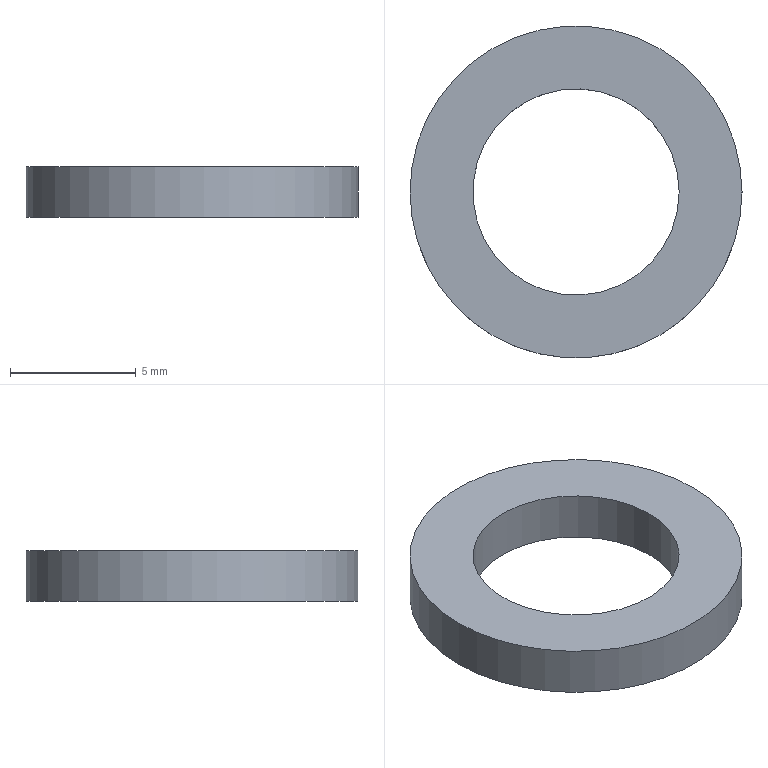Part | NX | features CYLINDER 2, DATUM_CSYS 1 | 1 solid | 4 faces | box 13.2 x 13.2 x 2 mm | volume 168.075 mm3 | plane 2 | cylinder 2 | commonest cylinder face diameters 8.2 x1 13.2 x1
STEP:
#1=CARTESIAN_POINT('',(4.1,0.,2.));
#2=VERTEX_POINT('',#1);
#3=CARTESIAN_POINT('',(0.,0.,2.));
#4=DIRECTION('',(0.,0.,-1.));
#5=DIRECTION('',(1.,0.,0.));
#6=AXIS2_PLACEMENT_3D('',#3,#4,#5);
#7=CIRCLE('',#6,4.1);
#8=EDGE_CURVE('',#2,#2,#7,.T.);
#9=ORIENTED_EDGE('',*,*,#8,.T.);
#10=EDGE_LOOP('',(#9));
#11=FACE_BOUND('',#10,.T.);
#12=CARTESIAN_POINT('',(6.6,0.,2.));
#13=VERTEX_POINT('',#12);
#14=CARTESIAN_POINT('',(0.,0.,2.));
#15=DIRECTION('',(0.,0.,-1.));
#16=DIRECTION('',(1.,0.,0.));
#17=AXIS2_PLACEMENT_3D('',#14,#15,#16);
#18=CIRCLE('',#17,6.6);
#19=EDGE_CURVE('',#13,#13,#18,.T.);
#20=ORIENTED_EDGE('',*,*,#19,.F.);
#21=EDGE_LOOP('',(#20));
#22=FACE_BOUND('',#21,.T.);
#23=CARTESIAN_POINT('',(0.,0.,2.));
#24=DIRECTION('',(0.,0.,1.));
#25=DIRECTION('',(1.,0.,0.));
#26=AXIS2_PLACEMENT_3D('',#23,#24,#25);
#27=PLANE('',#26);
#28=ADVANCED_FACE('',(#11,#22),#27,.T.);
#29=CARTESIAN_POINT('',(4.1,0.,0.));
#30=VERTEX_POINT('',#29);
#31=CARTESIAN_POINT('',(0.,0.,0.));
#32=DIRECTION('',(0.,0.,1.));
#33=DIRECTION('',(1.,0.,0.));
#34=AXIS2_PLACEMENT_3D('',#31,#32,#33);
#35=CIRCLE('',#34,4.1);
#36=EDGE_CURVE('',#30,#30,#35,.T.);
#37=ORIENTED_EDGE('',*,*,#36,.T.);
#38=EDGE_LOOP('',(#37));
#39=FACE_BOUND('',#38,.T.);
#40=CARTESIAN_POINT('',(6.6,0.,0.));
#41=VERTEX_POINT('',#40);
#42=CARTESIAN_POINT('',(0.,0.,0.));
#43=DIRECTION('',(0.,0.,1.));
#44=DIRECTION('',(1.,0.,0.));
#45=AXIS2_PLACEMENT_3D('',#42,#43,#44);
#46=CIRCLE('',#45,6.6);
#47=EDGE_CURVE('',#41,#41,#46,.T.);
#48=ORIENTED_EDGE('',*,*,#47,.F.);
#49=EDGE_LOOP('',(#48));
#50=FACE_BOUND('',#49,.T.);
#51=CARTESIAN_POINT('',(0.,0.,0.));
#52=DIRECTION('',(0.,0.,-1.));
#53=DIRECTION('',(-1.,0.,0.));
#54=AXIS2_PLACEMENT_3D('',#51,#52,#53);
#55=PLANE('',#54);
#56=ADVANCED_FACE('',(#39,#50),#55,.T.);
#57=ORIENTED_EDGE('',*,*,#19,.T.);
#58=EDGE_LOOP('',(#57));
#59=FACE_BOUND('',#58,.T.);
#60=ORIENTED_EDGE('',*,*,#47,.T.);
#61=EDGE_LOOP('',(#60));
#62=FACE_BOUND('',#61,.T.);
#63=CARTESIAN_POINT('',(0.,0.,0.));
#64=DIRECTION('',(0.,0.,1.));
#65=DIRECTION('',(1.,0.,0.));
#66=AXIS2_PLACEMENT_3D('',#63,#64,#65);
#67=CYLINDRICAL_SURFACE('',#66,6.6);
#68=ADVANCED_FACE('',(#59,#62),#67,.T.);
#69=ORIENTED_EDGE('',*,*,#8,.F.);
#70=EDGE_LOOP('',(#69));
#71=FACE_BOUND('',#70,.T.);
#72=ORIENTED_EDGE('',*,*,#36,.F.);
#73=EDGE_LOOP('',(#72));
#74=FACE_BOUND('',#73,.T.);
#75=CARTESIAN_POINT('',(0.,0.,0.));
#76=DIRECTION('',(0.,0.,1.));
#77=DIRECTION('',(1.,0.,0.));
#78=AXIS2_PLACEMENT_3D('',#75,#76,#77);
#79=CYLINDRICAL_SURFACE('',#78,4.1);
#80=ADVANCED_FACE('',(#71,#74),#79,.F.);
#81=CLOSED_SHELL('',(#28,#56,#68,#80));
#82=MANIFOLD_SOLID_BREP('',#81);
#83=(LENGTH_UNIT()NAMED_UNIT(*)SI_UNIT(.MILLI.,.METRE.));
#84=UNCERTAINTY_MEASURE_WITH_UNIT(LENGTH_MEASURE(0.00001),#83,'','');
#85=(NAMED_UNIT(*)PLANE_ANGLE_UNIT()SI_UNIT($,.RADIAN.));
#86=(NAMED_UNIT(*)SI_UNIT($,.STERADIAN.)SOLID_ANGLE_UNIT());
#87=(GEOMETRIC_REPRESENTATION_CONTEXT(3)GLOBAL_UNCERTAINTY_ASSIGNED_CONTEXT((#84))GLOBAL_UNIT_ASSIGNED_CONTEXT((#83,#85,#86))REPRESENTATION_CONTEXT('',''));
#88=ADVANCED_BREP_SHAPE_REPRESENTATION('',(#82),#87);